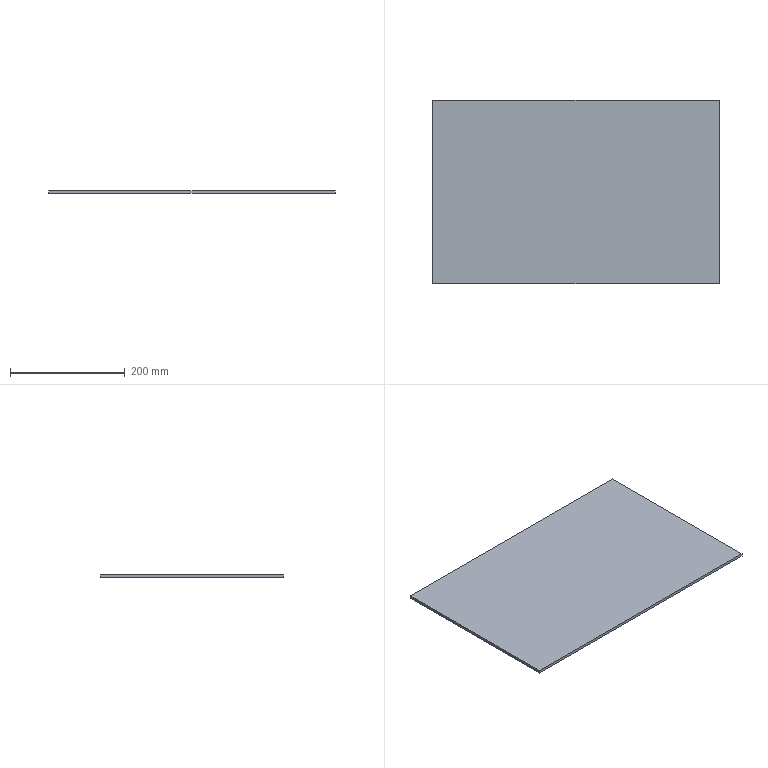Part | SolidWorks | features Extrusion 1 | 1 solid | 6 faces | box 500 x 320 x 5 mm | volume 800000 mm3 | plane 6
STEP:
#1=CARTESIAN_POINT('',(0.,320.,0.));
#2=VERTEX_POINT('',#1);
#3=CARTESIAN_POINT('',(0.,0.,0.));
#4=VERTEX_POINT('',#3);
#5=CARTESIAN_POINT('',(0.,0.,0.));
#6=DIRECTION('',(0.,-1.,0.));
#7=VECTOR('',#6,1000.);
#8=LINE('',#5,#7);
#9=EDGE_CURVE('',#2,#4,#8,.T.);
#10=ORIENTED_EDGE('',*,*,#9,.T.);
#11=CARTESIAN_POINT('',(0.,0.,5.));
#12=VERTEX_POINT('',#11);
#13=CARTESIAN_POINT('',(0.,0.,5.));
#14=DIRECTION('',(0.,0.,-1.));
#15=VECTOR('',#14,1000.);
#16=LINE('',#13,#15);
#17=EDGE_CURVE('',#12,#4,#16,.T.);
#18=ORIENTED_EDGE('',*,*,#17,.F.);
#19=CARTESIAN_POINT('',(0.,320.,5.));
#20=VERTEX_POINT('',#19);
#21=CARTESIAN_POINT('',(0.,0.,5.));
#22=DIRECTION('',(0.,-1.,0.));
#23=VECTOR('',#22,1000.);
#24=LINE('',#21,#23);
#25=EDGE_CURVE('',#20,#12,#24,.T.);
#26=ORIENTED_EDGE('',*,*,#25,.F.);
#27=CARTESIAN_POINT('',(0.,320.,5.));
#28=DIRECTION('',(0.,0.,-1.));
#29=VECTOR('',#28,1000.);
#30=LINE('',#27,#29);
#31=EDGE_CURVE('',#20,#2,#30,.T.);
#32=ORIENTED_EDGE('',*,*,#31,.T.);
#33=EDGE_LOOP('',(#10,#18,#26,#32));
#34=FACE_OUTER_BOUND('',#33,.T.);
#35=CARTESIAN_POINT('',(0.,0.,5.));
#36=DIRECTION('',(1.,0.,0.));
#37=DIRECTION('',(0.,0.,-1.));
#38=AXIS2_PLACEMENT_3D('',#35,#36,#37);
#39=PLANE('',#38);
#40=ADVANCED_FACE('',(#34),#39,.F.);
#41=CARTESIAN_POINT('',(500.,0.,0.));
#42=VERTEX_POINT('',#41);
#43=CARTESIAN_POINT('',(0.,0.,0.));
#44=DIRECTION('',(1.,0.,0.));
#45=VECTOR('',#44,1000.);
#46=LINE('',#43,#45);
#47=EDGE_CURVE('',#4,#42,#46,.T.);
#48=ORIENTED_EDGE('',*,*,#47,.T.);
#49=CARTESIAN_POINT('',(500.,0.,5.));
#50=VERTEX_POINT('',#49);
#51=CARTESIAN_POINT('',(500.,0.,5.));
#52=DIRECTION('',(0.,0.,-1.));
#53=VECTOR('',#52,1000.);
#54=LINE('',#51,#53);
#55=EDGE_CURVE('',#50,#42,#54,.T.);
#56=ORIENTED_EDGE('',*,*,#55,.F.);
#57=CARTESIAN_POINT('',(0.,0.,5.));
#58=DIRECTION('',(1.,0.,0.));
#59=VECTOR('',#58,1000.);
#60=LINE('',#57,#59);
#61=EDGE_CURVE('',#12,#50,#60,.T.);
#62=ORIENTED_EDGE('',*,*,#61,.F.);
#63=ORIENTED_EDGE('',*,*,#17,.T.);
#64=EDGE_LOOP('',(#48,#56,#62,#63));
#65=FACE_OUTER_BOUND('',#64,.T.);
#66=CARTESIAN_POINT('',(0.,0.,5.));
#67=DIRECTION('',(0.,1.,0.));
#68=DIRECTION('',(0.,0.,1.));
#69=AXIS2_PLACEMENT_3D('',#66,#67,#68);
#70=PLANE('',#69);
#71=ADVANCED_FACE('',(#65),#70,.F.);
#72=CARTESIAN_POINT('',(500.,320.,0.));
#73=VERTEX_POINT('',#72);
#74=CARTESIAN_POINT('',(500.,0.,0.));
#75=DIRECTION('',(0.,1.,0.));
#76=VECTOR('',#75,1000.);
#77=LINE('',#74,#76);
#78=EDGE_CURVE('',#42,#73,#77,.T.);
#79=ORIENTED_EDGE('',*,*,#78,.T.);
#80=CARTESIAN_POINT('',(500.,320.,5.));
#81=VERTEX_POINT('',#80);
#82=CARTESIAN_POINT('',(500.,320.,5.));
#83=DIRECTION('',(0.,0.,-1.));
#84=VECTOR('',#83,1000.);
#85=LINE('',#82,#84);
#86=EDGE_CURVE('',#81,#73,#85,.T.);
#87=ORIENTED_EDGE('',*,*,#86,.F.);
#88=CARTESIAN_POINT('',(500.,0.,5.));
#89=DIRECTION('',(0.,1.,0.));
#90=VECTOR('',#89,1000.);
#91=LINE('',#88,#90);
#92=EDGE_CURVE('',#50,#81,#91,.T.);
#93=ORIENTED_EDGE('',*,*,#92,.F.);
#94=ORIENTED_EDGE('',*,*,#55,.T.);
#95=EDGE_LOOP('',(#79,#87,#93,#94));
#96=FACE_OUTER_BOUND('',#95,.T.);
#97=CARTESIAN_POINT('',(500.,0.,5.));
#98=DIRECTION('',(-1.,0.,0.));
#99=DIRECTION('',(0.,0.,1.));
#100=AXIS2_PLACEMENT_3D('',#97,#98,#99);
#101=PLANE('',#100);
#102=ADVANCED_FACE('',(#96),#101,.F.);
#103=CARTESIAN_POINT('',(0.,320.,0.));
#104=DIRECTION('',(-1.,0.,0.));
#105=VECTOR('',#104,1000.);
#106=LINE('',#103,#105);
#107=EDGE_CURVE('',#73,#2,#106,.T.);
#108=ORIENTED_EDGE('',*,*,#107,.T.);
#109=ORIENTED_EDGE('',*,*,#31,.F.);
#110=CARTESIAN_POINT('',(0.,320.,5.));
#111=DIRECTION('',(-1.,0.,0.));
#112=VECTOR('',#111,1000.);
#113=LINE('',#110,#112);
#114=EDGE_CURVE('',#81,#20,#113,.T.);
#115=ORIENTED_EDGE('',*,*,#114,.F.);
#116=ORIENTED_EDGE('',*,*,#86,.T.);
#117=EDGE_LOOP('',(#108,#109,#115,#116));
#118=FACE_OUTER_BOUND('',#117,.T.);
#119=CARTESIAN_POINT('',(0.,320.,5.));
#120=DIRECTION('',(0.,-1.,0.));
#121=DIRECTION('',(0.,0.,-1.));
#122=AXIS2_PLACEMENT_3D('',#119,#120,#121);
#123=PLANE('',#122);
#124=ADVANCED_FACE('',(#118),#123,.F.);
#125=ORIENTED_EDGE('',*,*,#25,.T.);
#126=ORIENTED_EDGE('',*,*,#61,.T.);
#127=ORIENTED_EDGE('',*,*,#92,.T.);
#128=ORIENTED_EDGE('',*,*,#114,.T.);
#129=EDGE_LOOP('',(#125,#126,#127,#128));
#130=FACE_OUTER_BOUND('',#129,.T.);
#131=CARTESIAN_POINT('',(0.,0.,5.));
#132=DIRECTION('',(0.,0.,-1.));
#133=DIRECTION('',(-1.,0.,0.));
#134=AXIS2_PLACEMENT_3D('',#131,#132,#133);
#135=PLANE('',#134);
#136=ADVANCED_FACE('',(#130),#135,.F.);
#137=ORIENTED_EDGE('',*,*,#9,.F.);
#138=ORIENTED_EDGE('',*,*,#107,.F.);
#139=ORIENTED_EDGE('',*,*,#78,.F.);
#140=ORIENTED_EDGE('',*,*,#47,.F.);
#141=EDGE_LOOP('',(#137,#138,#139,#140));
#142=FACE_OUTER_BOUND('',#141,.T.);
#143=CARTESIAN_POINT('',(0.,0.,0.));
#144=DIRECTION('',(0.,0.,-1.));
#145=DIRECTION('',(-1.,0.,0.));
#146=AXIS2_PLACEMENT_3D('',#143,#144,#145);
#147=PLANE('',#146);
#148=ADVANCED_FACE('',(#142),#147,.T.);
#149=CLOSED_SHELL('',(#40,#71,#102,#124,#136,#148));
#150=MANIFOLD_SOLID_BREP('',#149);
#151=CARTESIAN_POINT('',(0.,0.,0.));
#152=DIRECTION('',(0.,0.,1.));
#153=DIRECTION('',(1.,0.,0.));
#154=AXIS2_PLACEMENT_3D('',#151,#152,#153);
#155=(LENGTH_UNIT()NAMED_UNIT(*)SI_UNIT(.MILLI.,.METRE.));
#156=UNCERTAINTY_MEASURE_WITH_UNIT(LENGTH_MEASURE(0.00001),#155,'','');
#157=(NAMED_UNIT(*)PLANE_ANGLE_UNIT()SI_UNIT($,.RADIAN.));
#158=(NAMED_UNIT(*)SI_UNIT($,.STERADIAN.)SOLID_ANGLE_UNIT());
#159=(GEOMETRIC_REPRESENTATION_CONTEXT(3)GLOBAL_UNCERTAINTY_ASSIGNED_CONTEXT((#156))GLOBAL_UNIT_ASSIGNED_CONTEXT((#155,#157,#158))REPRESENTATION_CONTEXT('',''));
#160=ADVANCED_BREP_SHAPE_REPRESENTATION('',(#150,#154),#159);